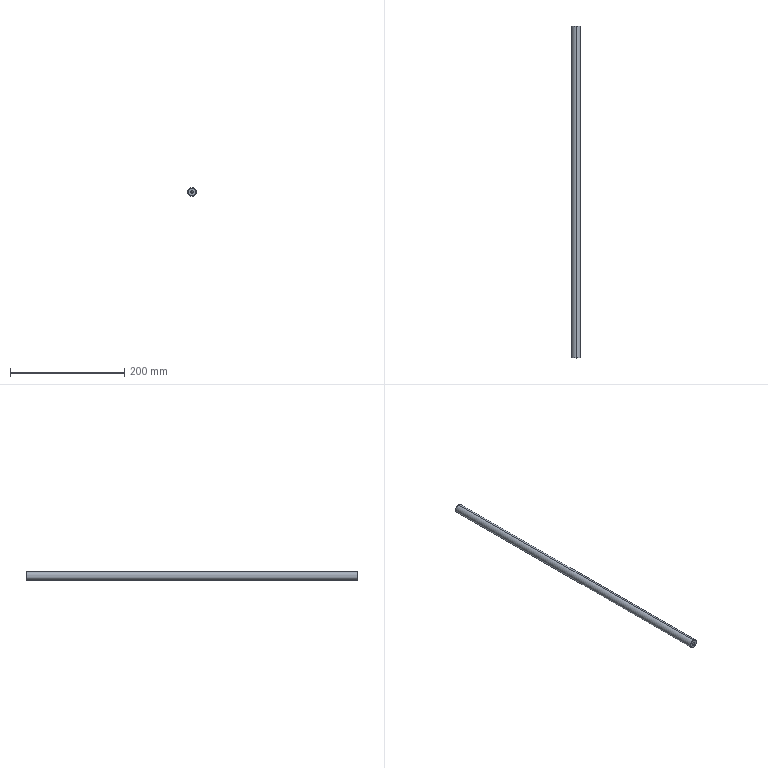Part | STEP file | PN_0005 | 1 solid | 16 faces | box 15 x 580 x 15 mm | volume 101796 mm3 | cone 8 | cylinder 6 | plane 2 | commonest cylinder face diameters 5 x4 15 x2
STEP:
#1=CARTESIAN_POINT('',(0.,0.,0.));
#2=DIRECTION('',(0.,0.,1.));
#3=DIRECTION('',(1.,0.,0.));
#4=AXIS2_PLACEMENT_3D('',#1,#2,#3);
#5=CARTESIAN_POINT('',(0.,580.,7.));
#6=VERTEX_POINT('',#5);
#7=CARTESIAN_POINT('',(0.,580.,-7.));
#8=VERTEX_POINT('',#7);
#9=CARTESIAN_POINT('',(0.,580.,0.));
#10=DIRECTION('',(0.,1.,0.));
#11=DIRECTION('',(0.,0.,1.));
#12=AXIS2_PLACEMENT_3D('',#9,#10,#11);
#13=CIRCLE('',#12,7.);
#14=CARTESIAN_POINT('',(0.,580.,0.));
#15=DIRECTION('',(0.,-1.,0.));
#16=DIRECTION('',(0.,0.,-1.));
#17=AXIS2_PLACEMENT_3D('',#14,#15,#16);
#18=CONICAL_SURFACE('',#17,7.,0.7854);
#19=CARTESIAN_POINT('',(3.142,0.));
#20=DIRECTION('',(-1.,0.));
#21=VECTOR('',#20,1.);
#22=LINE('',#19,#21);
#23=(GEOMETRIC_REPRESENTATION_CONTEXT(2)PARAMETRIC_REPRESENTATION_CONTEXT()REPRESENTATION_CONTEXT('',''));
#24=DEFINITIONAL_REPRESENTATION('',(#22),#23);
#25=PCURVE('',#18,#24);
#26=CARTESIAN_POINT('',(0.,580.,0.));
#27=DIRECTION('',(0.,1.,0.));
#28=DIRECTION('',(0.,0.,1.));
#29=AXIS2_PLACEMENT_3D('',#26,#27,#28);
#30=PLANE('',#29);
#31=CARTESIAN_POINT('',(0.,0.));
#32=DIRECTION('',(1.,0.));
#33=AXIS2_PLACEMENT_2D('',#31,#32);
#34=CIRCLE('',#33,7.);
#35=(GEOMETRIC_REPRESENTATION_CONTEXT(2)PARAMETRIC_REPRESENTATION_CONTEXT()REPRESENTATION_CONTEXT('',''));
#36=DEFINITIONAL_REPRESENTATION('',(#34),#35);
#37=PCURVE('',#30,#36);
#38=SURFACE_CURVE('',#13,(#25,#37),.PCURVE_S1.);
#39=EDGE_CURVE('',#6,#8,#38,.T.);
#40=ORIENTED_EDGE('',*,*,#39,.F.);
#41=CARTESIAN_POINT('',(0.,579.5,7.5));
#42=VERTEX_POINT('',#41);
#43=CARTESIAN_POINT('',(0.,580.,7.));
#44=DIRECTION('',(0.,-0.7071,0.7071));
#45=VECTOR('',#44,1.);
#46=LINE('',#43,#45);
#47=CARTESIAN_POINT('',(3.142,0.));
#48=DIRECTION('',(0.,1.));
#49=VECTOR('',#48,1.);
#50=LINE('',#47,#49);
#51=(GEOMETRIC_REPRESENTATION_CONTEXT(2)PARAMETRIC_REPRESENTATION_CONTEXT()REPRESENTATION_CONTEXT('',''));
#52=DEFINITIONAL_REPRESENTATION('',(#50),#51);
#53=PCURVE('',#18,#52);
#54=CARTESIAN_POINT('',(0.,580.,0.));
#55=DIRECTION('',(0.,-1.,0.));
#56=DIRECTION('',(0.,0.,-1.));
#57=AXIS2_PLACEMENT_3D('',#54,#55,#56);
#58=CONICAL_SURFACE('',#57,7.,0.7854);
#59=CARTESIAN_POINT('',(3.142,0.));
#60=DIRECTION('',(0.,1.));
#61=VECTOR('',#60,1.);
#62=LINE('',#59,#61);
#63=(GEOMETRIC_REPRESENTATION_CONTEXT(2)PARAMETRIC_REPRESENTATION_CONTEXT()REPRESENTATION_CONTEXT('',''));
#64=DEFINITIONAL_REPRESENTATION('',(#62),#63);
#65=PCURVE('',#58,#64);
#66=SURFACE_CURVE('',#46,(#53,#65),.PCURVE_S1.);
#67=EDGE_CURVE('',#6,#42,#66,.T.);
#68=ORIENTED_EDGE('',*,*,#67,.T.);
#69=CARTESIAN_POINT('',(0.,579.5,-7.5));
#70=VERTEX_POINT('',#69);
#71=CARTESIAN_POINT('',(0.,579.5,0.));
#72=DIRECTION('',(0.,-1.,0.));
#73=DIRECTION('',(0.,0.,1.));
#74=AXIS2_PLACEMENT_3D('',#71,#72,#73);
#75=CIRCLE('',#74,7.5);
#76=CARTESIAN_POINT('',(-3.142,0.5));
#77=DIRECTION('',(1.,0.));
#78=VECTOR('',#77,1.);
#79=LINE('',#76,#78);
#80=(GEOMETRIC_REPRESENTATION_CONTEXT(2)PARAMETRIC_REPRESENTATION_CONTEXT()REPRESENTATION_CONTEXT('',''));
#81=DEFINITIONAL_REPRESENTATION('',(#79),#80);
#82=PCURVE('',#18,#81);
#83=CARTESIAN_POINT('',(0.,580.,0.));
#84=DIRECTION('',(0.,-1.,0.));
#85=DIRECTION('',(0.,0.,-1.));
#86=AXIS2_PLACEMENT_3D('',#83,#84,#85);
#87=CYLINDRICAL_SURFACE('',#86,7.5);
#88=CARTESIAN_POINT('',(-3.142,0.5));
#89=DIRECTION('',(1.,0.));
#90=VECTOR('',#89,1.);
#91=LINE('',#88,#90);
#92=(GEOMETRIC_REPRESENTATION_CONTEXT(2)PARAMETRIC_REPRESENTATION_CONTEXT()REPRESENTATION_CONTEXT('',''));
#93=DEFINITIONAL_REPRESENTATION('',(#91),#92);
#94=PCURVE('',#87,#93);
#95=SURFACE_CURVE('',#75,(#82,#94),.PCURVE_S1.);
#96=EDGE_CURVE('',#70,#42,#95,.T.);
#97=ORIENTED_EDGE('',*,*,#96,.F.);
#98=CARTESIAN_POINT('',(0.,580.,-7.));
#99=DIRECTION('',(0.,-0.7071,-0.7071));
#100=VECTOR('',#99,1.);
#101=LINE('',#98,#100);
#102=CARTESIAN_POINT('',(0.,0.));
#103=DIRECTION('',(0.,1.));
#104=VECTOR('',#103,1.);
#105=LINE('',#102,#104);
#106=(GEOMETRIC_REPRESENTATION_CONTEXT(2)PARAMETRIC_REPRESENTATION_CONTEXT()REPRESENTATION_CONTEXT('',''));
#107=DEFINITIONAL_REPRESENTATION('',(#105),#106);
#108=PCURVE('',#18,#107);
#109=CARTESIAN_POINT('',(6.283,0.));
#110=DIRECTION('',(0.,1.));
#111=VECTOR('',#110,1.);
#112=LINE('',#109,#111);
#113=(GEOMETRIC_REPRESENTATION_CONTEXT(2)PARAMETRIC_REPRESENTATION_CONTEXT()REPRESENTATION_CONTEXT('',''));
#114=DEFINITIONAL_REPRESENTATION('',(#112),#113);
#115=PCURVE('',#58,#114);
#116=SURFACE_CURVE('',#101,(#108,#115),.PCURVE_S1.);
#117=EDGE_CURVE('',#8,#70,#116,.T.);
#118=ORIENTED_EDGE('',*,*,#117,.F.);
#119=EDGE_LOOP('',(#40,#68,#97,#118));
#120=FACE_BOUND('',#119,.T.);
#121=ADVANCED_FACE('',(#120),#18,.T.);
#122=CARTESIAN_POINT('',(0.,0.,-7.));
#123=VERTEX_POINT('',#122);
#124=CARTESIAN_POINT('',(0.,0.,7.));
#125=VERTEX_POINT('',#124);
#126=CARTESIAN_POINT('',(0.,0.,0.));
#127=DIRECTION('',(0.,-1.,0.));
#128=DIRECTION('',(0.,0.,1.));
#129=AXIS2_PLACEMENT_3D('',#126,#127,#128);
#130=CIRCLE('',#129,7.);
#131=CARTESIAN_POINT('',(0.,0.5,0.));
#132=DIRECTION('',(0.,1.,0.));
#133=DIRECTION('',(0.,0.,1.));
#134=AXIS2_PLACEMENT_3D('',#131,#132,#133);
#135=CONICAL_SURFACE('',#134,7.5,0.7854);
#136=CARTESIAN_POINT('',(6.283,-0.5));
#137=DIRECTION('',(-1.,0.));
#138=VECTOR('',#137,1.);
#139=LINE('',#136,#138);
#140=(GEOMETRIC_REPRESENTATION_CONTEXT(2)PARAMETRIC_REPRESENTATION_CONTEXT()REPRESENTATION_CONTEXT('',''));
#141=DEFINITIONAL_REPRESENTATION('',(#139),#140);
#142=PCURVE('',#135,#141);
#143=CARTESIAN_POINT('',(0.,0.,0.));
#144=DIRECTION('',(0.,1.,0.));
#145=DIRECTION('',(0.,0.,1.));
#146=AXIS2_PLACEMENT_3D('',#143,#144,#145);
#147=PLANE('',#146);
#148=CARTESIAN_POINT('',(7.,0.));
#149=CARTESIAN_POINT('',(7.,-12.124));
#150=CARTESIAN_POINT('',(-3.5,-6.062));
#151=CARTESIAN_POINT('',(-14.,0.));
#152=CARTESIAN_POINT('',(-3.5,6.062));
#153=CARTESIAN_POINT('',(7.,12.124));
#154=CARTESIAN_POINT('',(7.,0.));
#155=(BOUNDED_CURVE()B_SPLINE_CURVE(2,(#148,#149,#150,#151,#152,#153,#154),.UNSPECIFIED.,.T.,.F.)B_SPLINE_CURVE_WITH_KNOTS((1,2,2,2,2,1),(-2.094,0.,2.094,4.189,6.283,8.378),.UNSPECIFIED.)CURVE()GEOMETRIC_REPRESENTATION_ITEM()RATIONAL_B_SPLINE_CURVE((1.,0.5,1.,0.5,1.,0.5,1.))REPRESENTATION_ITEM(''));
#156=(GEOMETRIC_REPRESENTATION_CONTEXT(2)PARAMETRIC_REPRESENTATION_CONTEXT()REPRESENTATION_CONTEXT('',''));
#157=DEFINITIONAL_REPRESENTATION('',(#155),#156);
#158=PCURVE('',#147,#157);
#159=SURFACE_CURVE('',#130,(#142,#158),.PCURVE_S1.);
#160=EDGE_CURVE('',#123,#125,#159,.T.);
#161=ORIENTED_EDGE('',*,*,#160,.F.);
#162=CARTESIAN_POINT('',(0.,0.5,-7.5));
#163=VERTEX_POINT('',#162);
#164=CARTESIAN_POINT('',(0.,0.5,-7.5));
#165=DIRECTION('',(0.,0.7071,-0.7071));
#166=VECTOR('',#165,1.);
#167=LINE('',#164,#166);
#168=CARTESIAN_POINT('',(3.142,0.));
#169=DIRECTION('',(0.,1.));
#170=VECTOR('',#169,1.);
#171=LINE('',#168,#170);
#172=(GEOMETRIC_REPRESENTATION_CONTEXT(2)PARAMETRIC_REPRESENTATION_CONTEXT()REPRESENTATION_CONTEXT('',''));
#173=DEFINITIONAL_REPRESENTATION('',(#171),#172);
#174=PCURVE('',#135,#173);
#175=CARTESIAN_POINT('',(0.,0.5,0.));
#176=DIRECTION('',(0.,1.,0.));
#177=DIRECTION('',(0.,0.,1.));
#178=AXIS2_PLACEMENT_3D('',#175,#176,#177);
#179=CONICAL_SURFACE('',#178,7.5,0.7854);
#180=CARTESIAN_POINT('',(3.142,0.));
#181=DIRECTION('',(0.,1.));
#182=VECTOR('',#181,1.);
#183=LINE('',#180,#182);
#184=(GEOMETRIC_REPRESENTATION_CONTEXT(2)PARAMETRIC_REPRESENTATION_CONTEXT()REPRESENTATION_CONTEXT('',''));
#185=DEFINITIONAL_REPRESENTATION('',(#183),#184);
#186=PCURVE('',#179,#185);
#187=SURFACE_CURVE('',#167,(#174,#186),.PCURVE_S1.);
#188=EDGE_CURVE('',#123,#163,#187,.T.);
#189=ORIENTED_EDGE('',*,*,#188,.T.);
#190=CARTESIAN_POINT('',(0.,0.5,7.5));
#191=VERTEX_POINT('',#190);
#192=CARTESIAN_POINT('',(0.,0.5,0.));
#193=DIRECTION('',(0.,1.,0.));
#194=DIRECTION('',(0.,0.,1.));
#195=AXIS2_PLACEMENT_3D('',#192,#193,#194);
#196=CIRCLE('',#195,7.5);
#197=CARTESIAN_POINT('',(0.,0.));
#198=DIRECTION('',(1.,0.));
#199=VECTOR('',#198,1.);
#200=LINE('',#197,#199);
#201=(GEOMETRIC_REPRESENTATION_CONTEXT(2)PARAMETRIC_REPRESENTATION_CONTEXT()REPRESENTATION_CONTEXT('',''));
#202=DEFINITIONAL_REPRESENTATION('',(#200),#201);
#203=PCURVE('',#135,#202);
#204=CARTESIAN_POINT('',(3.142,579.5));
#205=DIRECTION('',(-1.,0.));
#206=VECTOR('',#205,1.);
#207=LINE('',#204,#206);
#208=(GEOMETRIC_REPRESENTATION_CONTEXT(2)PARAMETRIC_REPRESENTATION_CONTEXT()REPRESENTATION_CONTEXT('',''));
#209=DEFINITIONAL_REPRESENTATION('',(#207),#208);
#210=PCURVE('',#87,#209);
#211=SURFACE_CURVE('',#196,(#203,#210),.PCURVE_S1.);
#212=EDGE_CURVE('',#191,#163,#211,.T.);
#213=ORIENTED_EDGE('',*,*,#212,.F.);
#214=CARTESIAN_POINT('',(0.,0.5,7.5));
#215=DIRECTION('',(0.,0.7071,0.7071));
#216=VECTOR('',#215,1.);
#217=LINE('',#214,#216);
#218=CARTESIAN_POINT('',(0.,0.));
#219=DIRECTION('',(0.,1.));
#220=VECTOR('',#219,1.);
#221=LINE('',#218,#220);
#222=(GEOMETRIC_REPRESENTATION_CONTEXT(2)PARAMETRIC_REPRESENTATION_CONTEXT()REPRESENTATION_CONTEXT('',''));
#223=DEFINITIONAL_REPRESENTATION('',(#221),#222);
#224=PCURVE('',#135,#223);
#225=CARTESIAN_POINT('',(6.283,0.));
#226=DIRECTION('',(0.,1.));
#227=VECTOR('',#226,1.);
#228=LINE('',#225,#227);
#229=(GEOMETRIC_REPRESENTATION_CONTEXT(2)PARAMETRIC_REPRESENTATION_CONTEXT()REPRESENTATION_CONTEXT('',''));
#230=DEFINITIONAL_REPRESENTATION('',(#228),#229);
#231=PCURVE('',#179,#230);
#232=SURFACE_CURVE('',#217,(#224,#231),.PCURVE_S1.);
#233=EDGE_CURVE('',#125,#191,#232,.T.);
#234=ORIENTED_EDGE('',*,*,#233,.F.);
#235=EDGE_LOOP('',(#161,#189,#213,#234));
#236=FACE_BOUND('',#235,.T.);
#237=ADVANCED_FACE('',(#236),#135,.T.);
#238=CARTESIAN_POINT('',(0.,563.,2.5));
#239=VERTEX_POINT('',#238);
#240=CARTESIAN_POINT('',(0.,580.,2.5));
#241=VERTEX_POINT('',#240);
#242=CARTESIAN_POINT('',(0.,580.,2.5));
#243=DIRECTION('',(0.,1.,0.));
#244=VECTOR('',#243,1.);
#245=LINE('',#242,#244);
#246=CARTESIAN_POINT('',(0.,580.,0.));
#247=DIRECTION('',(0.,1.,0.));
#248=DIRECTION('',(0.,0.,1.));
#249=AXIS2_PLACEMENT_3D('',#246,#247,#248);
#250=CYLINDRICAL_SURFACE('',#249,2.5);
#251=CARTESIAN_POINT('',(6.283,0.));
#252=DIRECTION('',(0.,1.));
#253=VECTOR('',#252,1.);
#254=LINE('',#251,#253);
#255=(GEOMETRIC_REPRESENTATION_CONTEXT(2)PARAMETRIC_REPRESENTATION_CONTEXT()REPRESENTATION_CONTEXT('',''));
#256=DEFINITIONAL_REPRESENTATION('',(#254),#255);
#257=PCURVE('',#250,#256);
#258=CARTESIAN_POINT('',(0.,580.,0.));
#259=DIRECTION('',(0.,1.,0.));
#260=DIRECTION('',(0.,0.,1.));
#261=AXIS2_PLACEMENT_3D('',#258,#259,#260);
#262=CYLINDRICAL_SURFACE('',#261,2.5);
#263=CARTESIAN_POINT('',(0.,0.));
#264=DIRECTION('',(0.,1.));
#265=VECTOR('',#264,1.);
#266=LINE('',#263,#265);
#267=(GEOMETRIC_REPRESENTATION_CONTEXT(2)PARAMETRIC_REPRESENTATION_CONTEXT()REPRESENTATION_CONTEXT('',''));
#268=DEFINITIONAL_REPRESENTATION('',(#266),#267);
#269=PCURVE('',#262,#268);
#270=SURFACE_CURVE('',#245,(#257,#269),.PCURVE_S1.);
#271=EDGE_CURVE('',#239,#241,#270,.T.);
#272=ORIENTED_EDGE('',*,*,#271,.T.);
#273=CARTESIAN_POINT('',(0.,580.,-2.5));
#274=VERTEX_POINT('',#273);
#275=CARTESIAN_POINT('',(0.,580.,0.));
#276=DIRECTION('',(0.,1.,0.));
#277=DIRECTION('',(0.,0.,1.));
#278=AXIS2_PLACEMENT_3D('',#275,#276,#277);
#279=CIRCLE('',#278,2.5);
#280=CARTESIAN_POINT('',(0.,0.));
#281=DIRECTION('',(1.,0.));
#282=VECTOR('',#281,1.);
#283=LINE('',#280,#282);
#284=(GEOMETRIC_REPRESENTATION_CONTEXT(2)PARAMETRIC_REPRESENTATION_CONTEXT()REPRESENTATION_CONTEXT('',''));
#285=DEFINITIONAL_REPRESENTATION('',(#283),#284);
#286=PCURVE('',#250,#285);
#287=CARTESIAN_POINT('',(0.,0.));
#288=DIRECTION('',(1.,0.));
#289=AXIS2_PLACEMENT_2D('',#287,#288);
#290=CIRCLE('',#289,2.5);
#291=(GEOMETRIC_REPRESENTATION_CONTEXT(2)PARAMETRIC_REPRESENTATION_CONTEXT()REPRESENTATION_CONTEXT('',''));
#292=DEFINITIONAL_REPRESENTATION('',(#290),#291);
#293=PCURVE('',#30,#292);
#294=SURFACE_CURVE('',#279,(#286,#293),.PCURVE_S1.);
#295=EDGE_CURVE('',#274,#241,#294,.T.);
#296=ORIENTED_EDGE('',*,*,#295,.F.);
#297=CARTESIAN_POINT('',(0.,563.,-2.5));
#298=VERTEX_POINT('',#297);
#299=CARTESIAN_POINT('',(0.,580.,-2.5));
#300=DIRECTION('',(0.,1.,0.));
#301=VECTOR('',#300,1.);
#302=LINE('',#299,#301);
#303=CARTESIAN_POINT('',(3.142,0.));
#304=DIRECTION('',(0.,1.));
#305=VECTOR('',#304,1.);
#306=LINE('',#303,#305);
#307=(GEOMETRIC_REPRESENTATION_CONTEXT(2)PARAMETRIC_REPRESENTATION_CONTEXT()REPRESENTATION_CONTEXT('',''));
#308=DEFINITIONAL_REPRESENTATION('',(#306),#307);
#309=PCURVE('',#250,#308);
#310=CARTESIAN_POINT('',(3.142,0.));
#311=DIRECTION('',(0.,1.));
#312=VECTOR('',#311,1.);
#313=LINE('',#310,#312);
#314=(GEOMETRIC_REPRESENTATION_CONTEXT(2)PARAMETRIC_REPRESENTATION_CONTEXT()REPRESENTATION_CONTEXT('',''));
#315=DEFINITIONAL_REPRESENTATION('',(#313),#314);
#316=PCURVE('',#262,#315);
#317=SURFACE_CURVE('',#302,(#309,#316),.PCURVE_S1.);
#318=EDGE_CURVE('',#298,#274,#317,.T.);
#319=ORIENTED_EDGE('',*,*,#318,.F.);
#320=CARTESIAN_POINT('',(0.,563.,0.));
#321=DIRECTION('',(0.,1.,0.));
#322=DIRECTION('',(0.,0.,1.));
#323=AXIS2_PLACEMENT_3D('',#320,#321,#322);
#324=CIRCLE('',#323,2.5);
#325=CARTESIAN_POINT('',(0.,-17.));
#326=DIRECTION('',(1.,0.));
#327=VECTOR('',#326,1.);
#328=LINE('',#325,#327);
#329=(GEOMETRIC_REPRESENTATION_CONTEXT(2)PARAMETRIC_REPRESENTATION_CONTEXT()REPRESENTATION_CONTEXT('',''));
#330=DEFINITIONAL_REPRESENTATION('',(#328),#329);
#331=PCURVE('',#250,#330);
#332=CARTESIAN_POINT('',(0.,563.,0.));
#333=DIRECTION('',(0.,1.,0.));
#334=DIRECTION('',(0.,0.,1.));
#335=AXIS2_PLACEMENT_3D('',#332,#333,#334);
#336=CONICAL_SURFACE('',#335,2.5,1.03);
#337=CARTESIAN_POINT('',(0.,0.));
#338=DIRECTION('',(1.,0.));
#339=VECTOR('',#338,1.);
#340=LINE('',#337,#339);
#341=(GEOMETRIC_REPRESENTATION_CONTEXT(2)PARAMETRIC_REPRESENTATION_CONTEXT()REPRESENTATION_CONTEXT('',''));
#342=DEFINITIONAL_REPRESENTATION('',(#340),#341);
#343=PCURVE('',#336,#342);
#344=SURFACE_CURVE('',#324,(#331,#343),.PCURVE_S1.);
#345=EDGE_CURVE('',#298,#239,#344,.T.);
#346=ORIENTED_EDGE('',*,*,#345,.T.);
#347=EDGE_LOOP('',(#272,#296,#319,#346));
#348=FACE_BOUND('',#347,.F.);
#349=ADVANCED_FACE('',(#348),#250,.F.);
#350=ORIENTED_EDGE('',*,*,#345,.F.);
#351=CARTESIAN_POINT('',(0.,561.498,0.));
#352=VERTEX_POINT('',#351);
#353=CARTESIAN_POINT('',(0.,563.,-2.5));
#354=DIRECTION('',(0.,0.515,-0.8572));
#355=VECTOR('',#354,1.);
#356=LINE('',#353,#355);
#357=CARTESIAN_POINT('',(3.142,-1.502));
#358=CARTESIAN_POINT('',(3.142,-1.479));
#359=CARTESIAN_POINT('',(3.142,-1.434));
#360=CARTESIAN_POINT('',(3.142,-1.366));
#361=CARTESIAN_POINT('',(3.142,-1.297));
#362=CARTESIAN_POINT('',(3.142,-1.229));
#363=CARTESIAN_POINT('',(3.142,-1.161));
#364=CARTESIAN_POINT('',(3.142,-1.092));
#365=CARTESIAN_POINT('',(3.142,-1.024));
#366=CARTESIAN_POINT('',(3.142,-0.9559));
#367=CARTESIAN_POINT('',(3.142,-0.8876));
#368=CARTESIAN_POINT('',(3.142,-0.8194));
#369=CARTESIAN_POINT('',(3.142,-0.7511));
#370=CARTESIAN_POINT('',(3.142,-0.6828));
#371=CARTESIAN_POINT('',(3.142,-0.6145));
#372=CARTESIAN_POINT('',(3.142,-0.5462));
#373=CARTESIAN_POINT('',(3.142,-0.478));
#374=CARTESIAN_POINT('',(3.142,-0.4097));
#375=CARTESIAN_POINT('',(3.142,-0.3414));
#376=CARTESIAN_POINT('',(3.142,-0.2731));
#377=CARTESIAN_POINT('',(3.142,-0.2048));
#378=CARTESIAN_POINT('',(3.142,-0.1366));
#379=CARTESIAN_POINT('',(3.142,-0.06828));
#380=CARTESIAN_POINT('',(3.142,-0.02276));
#381=CARTESIAN_POINT('',(3.142,0.));
#382=B_SPLINE_CURVE_WITH_KNOTS('',3,(#357,#358,#359,#360,#361,#362,#363,#364,#365,#366,#367,#368,#369,#370,#371,#372,#373,#374,#375,#376,#377,#378,#379,#380,#381),.UNSPECIFIED.,.F.,.F.,(4,1,1,1,1,1,1,1,1,1,1,1,1,1,1,1,1,1,1,1,1,1,4),(-2.917,-2.784,-2.651,-2.519,-2.386,-2.254,-2.121,-1.989,-1.856,-1.723,-1.591,-1.458,-1.326,-1.193,-1.061,-0.928,-0.7954,-0.6629,-0.5303,-0.3977,-0.2651,-0.1326,0.),.UNSPECIFIED.);
#383=(GEOMETRIC_REPRESENTATION_CONTEXT(2)PARAMETRIC_REPRESENTATION_CONTEXT()REPRESENTATION_CONTEXT('',''));
#384=DEFINITIONAL_REPRESENTATION('',(#382),#383);
#385=PCURVE('',#336,#384);
#386=CARTESIAN_POINT('',(0.,563.,0.));
#387=DIRECTION('',(0.,1.,0.));
#388=DIRECTION('',(0.,0.,1.));
#389=AXIS2_PLACEMENT_3D('',#386,#387,#388);
#390=CONICAL_SURFACE('',#389,2.5,1.03);
#391=CARTESIAN_POINT('',(3.142,-1.502));
#392=CARTESIAN_POINT('',(3.142,-1.479));
#393=CARTESIAN_POINT('',(3.142,-1.434));
#394=CARTESIAN_POINT('',(3.142,-1.366));
#395=CARTESIAN_POINT('',(3.142,-1.297));
#396=CARTESIAN_POINT('',(3.142,-1.229));
#397=CARTESIAN_POINT('',(3.142,-1.161));
#398=CARTESIAN_POINT('',(3.142,-1.092));
#399=CARTESIAN_POINT('',(3.142,-1.024));
#400=CARTESIAN_POINT('',(3.142,-0.9559));
#401=CARTESIAN_POINT('',(3.142,-0.8876));
#402=CARTESIAN_POINT('',(3.142,-0.8194));
#403=CARTESIAN_POINT('',(3.142,-0.7511));
#404=CARTESIAN_POINT('',(3.142,-0.6828));
#405=CARTESIAN_POINT('',(3.142,-0.6145));
#406=CARTESIAN_POINT('',(3.142,-0.5462));
#407=CARTESIAN_POINT('',(3.142,-0.478));
#408=CARTESIAN_POINT('',(3.142,-0.4097));
#409=CARTESIAN_POINT('',(3.142,-0.3414));
#410=CARTESIAN_POINT('',(3.142,-0.2731));
#411=CARTESIAN_POINT('',(3.142,-0.2048));
#412=CARTESIAN_POINT('',(3.142,-0.1366));
#413=CARTESIAN_POINT('',(3.142,-0.06828));
#414=CARTESIAN_POINT('',(3.142,-0.02276));
#415=CARTESIAN_POINT('',(3.142,0.));
#416=B_SPLINE_CURVE_WITH_KNOTS('',3,(#391,#392,#393,#394,#395,#396,#397,#398,#399,#400,#401,#402,#403,#404,#405,#406,#407,#408,#409,#410,#411,#412,#413,#414,#415),.UNSPECIFIED.,.F.,.F.,(4,1,1,1,1,1,1,1,1,1,1,1,1,1,1,1,1,1,1,1,1,1,4),(-2.917,-2.784,-2.651,-2.519,-2.386,-2.254,-2.121,-1.989,-1.856,-1.723,-1.591,-1.458,-1.326,-1.193,-1.061,-0.928,-0.7954,-0.6629,-0.5303,-0.3977,-0.2651,-0.1326,0.),.UNSPECIFIED.);
#417=(GEOMETRIC_REPRESENTATION_CONTEXT(2)PARAMETRIC_REPRESENTATION_CONTEXT()REPRESENTATION_CONTEXT('',''));
#418=DEFINITIONAL_REPRESENTATION('',(#416),#417);
#419=PCURVE('',#390,#418);
#420=SURFACE_CURVE('',#356,(#385,#419),.PCURVE_S1.);
#421=EDGE_CURVE('',#352,#298,#420,.T.);
#422=ORIENTED_EDGE('',*,*,#421,.F.);
#423=CARTESIAN_POINT('',(0.,563.,2.5));
#424=DIRECTION('',(0.,0.515,0.8572));
#425=VECTOR('',#424,1.);
#426=LINE('',#423,#425);
#427=CARTESIAN_POINT('',(6.283,-1.502));
#428=CARTESIAN_POINT('',(6.283,-1.479));
#429=CARTESIAN_POINT('',(6.283,-1.434));
#430=CARTESIAN_POINT('',(6.283,-1.366));
#431=CARTESIAN_POINT('',(6.283,-1.297));
#432=CARTESIAN_POINT('',(6.283,-1.229));
#433=CARTESIAN_POINT('',(6.283,-1.161));
#434=CARTESIAN_POINT('',(6.283,-1.092));
#435=CARTESIAN_POINT('',(6.283,-1.024));
#436=CARTESIAN_POINT('',(6.283,-0.9559));
#437=CARTESIAN_POINT('',(6.283,-0.8876));
#438=CARTESIAN_POINT('',(6.283,-0.8194));
#439=CARTESIAN_POINT('',(6.283,-0.7511));
#440=CARTESIAN_POINT('',(6.283,-0.6828));
#441=CARTESIAN_POINT('',(6.283,-0.6145));
#442=CARTESIAN_POINT('',(6.283,-0.5462));
#443=CARTESIAN_POINT('',(6.283,-0.478));
#444=CARTESIAN_POINT('',(6.283,-0.4097));
#445=CARTESIAN_POINT('',(6.283,-0.3414));
#446=CARTESIAN_POINT('',(6.283,-0.2731));
#447=CARTESIAN_POINT('',(6.283,-0.2048));
#448=CARTESIAN_POINT('',(6.283,-0.1366));
#449=CARTESIAN_POINT('',(6.283,-0.06828));
#450=CARTESIAN_POINT('',(6.283,-0.02276));
#451=CARTESIAN_POINT('',(6.283,0.));
#452=B_SPLINE_CURVE_WITH_KNOTS('',3,(#427,#428,#429,#430,#431,#432,#433,#434,#435,#436,#437,#438,#439,#440,#441,#442,#443,#444,#445,#446,#447,#448,#449,#450,#451),.UNSPECIFIED.,.F.,.F.,(4,1,1,1,1,1,1,1,1,1,1,1,1,1,1,1,1,1,1,1,1,1,4),(-2.917,-2.784,-2.651,-2.519,-2.386,-2.254,-2.121,-1.989,-1.856,-1.723,-1.591,-1.458,-1.326,-1.193,-1.061,-0.928,-0.7954,-0.6629,-0.5303,-0.3977,-0.2651,-0.1326,0.),.UNSPECIFIED.);
#453=(GEOMETRIC_REPRESENTATION_CONTEXT(2)PARAMETRIC_REPRESENTATION_CONTEXT()REPRESENTATION_CONTEXT('',''));
#454=DEFINITIONAL_REPRESENTATION('',(#452),#453);
#455=PCURVE('',#336,#454);
#456=CARTESIAN_POINT('',(0.,-1.502));
#457=CARTESIAN_POINT('',(0.,-1.479));
#458=CARTESIAN_POINT('',(0.,-1.434));
#459=CARTESIAN_POINT('',(0.,-1.366));
#460=CARTESIAN_POINT('',(0.,-1.297));
#461=CARTESIAN_POINT('',(0.,-1.229));
#462=CARTESIAN_POINT('',(0.,-1.161));
#463=CARTESIAN_POINT('',(0.,-1.092));
#464=CARTESIAN_POINT('',(0.,-1.024));
#465=CARTESIAN_POINT('',(0.,-0.9559));
#466=CARTESIAN_POINT('',(0.,-0.8876));
#467=CARTESIAN_POINT('',(0.,-0.8194));
#468=CARTESIAN_POINT('',(0.,-0.7511));
#469=CARTESIAN_POINT('',(0.,-0.6828));
#470=CARTESIAN_POINT('',(0.,-0.6145));
#471=CARTESIAN_POINT('',(0.,-0.5462));
#472=CARTESIAN_POINT('',(0.,-0.478));
#473=CARTESIAN_POINT('',(0.,-0.4097));
#474=CARTESIAN_POINT('',(0.,-0.3414));
#475=CARTESIAN_POINT('',(0.,-0.2731));
#476=CARTESIAN_POINT('',(0.,-0.2048));
#477=CARTESIAN_POINT('',(0.,-0.1366));
#478=CARTESIAN_POINT('',(0.,-0.06828));
#479=CARTESIAN_POINT('',(0.,-0.02276));
#480=CARTESIAN_POINT('',(0.,0.));
#481=B_SPLINE_CURVE_WITH_KNOTS('',3,(#456,#457,#458,#459,#460,#461,#462,#463,#464,#465,#466,#467,#468,#469,#470,#471,#472,#473,#474,#475,#476,#477,#478,#479,#480),.UNSPECIFIED.,.F.,.F.,(4,1,1,1,1,1,1,1,1,1,1,1,1,1,1,1,1,1,1,1,1,1,4),(-2.917,-2.784,-2.651,-2.519,-2.386,-2.254,-2.121,-1.989,-1.856,-1.723,-1.591,-1.458,-1.326,-1.193,-1.061,-0.928,-0.7954,-0.6629,-0.5303,-0.3977,-0.2651,-0.1326,0.),.UNSPECIFIED.);
#482=(GEOMETRIC_REPRESENTATION_CONTEXT(2)PARAMETRIC_REPRESENTATION_CONTEXT()REPRESENTATION_CONTEXT('',''));
#483=DEFINITIONAL_REPRESENTATION('',(#481),#482);
#484=PCURVE('',#390,#483);
#485=SURFACE_CURVE('',#426,(#455,#484),.PCURVE_S1.);
#486=EDGE_CURVE('',#352,#239,#485,.T.);
#487=ORIENTED_EDGE('',*,*,#486,.T.);
#488=EDGE_LOOP('',(#350,#422,#487));
#489=FACE_BOUND('',#488,.F.);
#490=ADVANCED_FACE('',(#489),#336,.F.);
#491=CARTESIAN_POINT('',(0.,17.,-2.5));
#492=VERTEX_POINT('',#491);
#493=CARTESIAN_POINT('',(0.,0.,-2.5));
#494=VERTEX_POINT('',#493);
#495=CARTESIAN_POINT('',(0.,0.,-2.5));
#496=DIRECTION('',(0.,-1.,0.));
#497=VECTOR('',#496,1.);
#498=LINE('',#495,#497);
#499=CARTESIAN_POINT('',(0.,0.,0.));
#500=DIRECTION('',(0.,-1.,0.));
#501=DIRECTION('',(0.,0.,-1.));
#502=AXIS2_PLACEMENT_3D('',#499,#500,#501);
#503=CYLINDRICAL_SURFACE('',#502,2.5);
#504=CARTESIAN_POINT('',(6.283,0.));
#505=DIRECTION('',(0.,1.));
#506=VECTOR('',#505,1.);
#507=LINE('',#504,#506);
#508=(GEOMETRIC_REPRESENTATION_CONTEXT(2)PARAMETRIC_REPRESENTATION_CONTEXT()REPRESENTATION_CONTEXT('',''));
#509=DEFINITIONAL_REPRESENTATION('',(#507),#508);
#510=PCURVE('',#503,#509);
#511=CARTESIAN_POINT('',(0.,0.,0.));
#512=DIRECTION('',(0.,-1.,0.));
#513=DIRECTION('',(0.,0.,-1.));
#514=AXIS2_PLACEMENT_3D('',#511,#512,#513);
#515=CYLINDRICAL_SURFACE('',#514,2.5);
#516=CARTESIAN_POINT('',(0.,0.));
#517=DIRECTION('',(0.,1.));
#518=VECTOR('',#517,1.);
#519=LINE('',#516,#518);
#520=(GEOMETRIC_REPRESENTATION_CONTEXT(2)PARAMETRIC_REPRESENTATION_CONTEXT()REPRESENTATION_CONTEXT('',''));
#521=DEFINITIONAL_REPRESENTATION('',(#519),#520);
#522=PCURVE('',#515,#521);
#523=SURFACE_CURVE('',#498,(#510,#522),.PCURVE_S1.);
#524=EDGE_CURVE('',#492,#494,#523,.T.);
#525=ORIENTED_EDGE('',*,*,#524,.T.);
#526=CARTESIAN_POINT('',(0.,0.,2.5));
#527=VERTEX_POINT('',#526);
#528=CARTESIAN_POINT('',(0.,0.,0.));
#529=DIRECTION('',(0.,-1.,0.));
#530=DIRECTION('',(0.,0.,-1.));
#531=AXIS2_PLACEMENT_3D('',#528,#529,#530);
#532=CIRCLE('',#531,2.5);
#533=CARTESIAN_POINT('',(0.,0.));
#534=DIRECTION('',(1.,0.));
#535=VECTOR('',#534,1.);
#536=LINE('',#533,#535);
#537=(GEOMETRIC_REPRESENTATION_CONTEXT(2)PARAMETRIC_REPRESENTATION_CONTEXT()REPRESENTATION_CONTEXT('',''));
#538=DEFINITIONAL_REPRESENTATION('',(#536),#537);
#539=PCURVE('',#503,#538);
#540=CARTESIAN_POINT('',(-2.5,0.));
#541=CARTESIAN_POINT('',(-2.5,4.33));
#542=CARTESIAN_POINT('',(1.25,2.165));
#543=CARTESIAN_POINT('',(5.,0.));
#544=CARTESIAN_POINT('',(1.25,-2.165));
#545=CARTESIAN_POINT('',(-2.5,-4.33));
#546=CARTESIAN_POINT('',(-2.5,0.));
#547=(BOUNDED_CURVE()B_SPLINE_CURVE(2,(#540,#541,#542,#543,#544,#545,#546),.UNSPECIFIED.,.T.,.F.)B_SPLINE_CURVE_WITH_KNOTS((1,2,2,2,2,1),(-2.094,0.,2.094,4.189,6.283,8.378),.UNSPECIFIED.)CURVE()GEOMETRIC_REPRESENTATION_ITEM()RATIONAL_B_SPLINE_CURVE((1.,0.5,1.,0.5,1.,0.5,1.))REPRESENTATION_ITEM(''));
#548=(GEOMETRIC_REPRESENTATION_CONTEXT(2)PARAMETRIC_REPRESENTATION_CONTEXT()REPRESENTATION_CONTEXT('',''));
#549=DEFINITIONAL_REPRESENTATION('',(#547),#548);
#550=PCURVE('',#147,#549);
#551=SURFACE_CURVE('',#532,(#539,#550),.PCURVE_S1.);
#552=EDGE_CURVE('',#527,#494,#551,.T.);
#553=ORIENTED_EDGE('',*,*,#552,.F.);
#554=CARTESIAN_POINT('',(0.,17.,2.5));
#555=VERTEX_POINT('',#554);
#556=CARTESIAN_POINT('',(0.,0.,2.5));
#557=DIRECTION('',(0.,-1.,0.));
#558=VECTOR('',#557,1.);
#559=LINE('',#556,#558);
#560=CARTESIAN_POINT('',(3.142,0.));
#561=DIRECTION('',(0.,1.));
#562=VECTOR('',#561,1.);
#563=LINE('',#560,#562);
#564=(GEOMETRIC_REPRESENTATION_CONTEXT(2)PARAMETRIC_REPRESENTATION_CONTEXT()REPRESENTATION_CONTEXT('',''));
#565=DEFINITIONAL_REPRESENTATION('',(#563),#564);
#566=PCURVE('',#503,#565);
#567=CARTESIAN_POINT('',(3.142,0.));
#568=DIRECTION('',(0.,1.));
#569=VECTOR('',#568,1.);
#570=LINE('',#567,#569);
#571=(GEOMETRIC_REPRESENTATION_CONTEXT(2)PARAMETRIC_REPRESENTATION_CONTEXT()REPRESENTATION_CONTEXT('',''));
#572=DEFINITIONAL_REPRESENTATION('',(#570),#571);
#573=PCURVE('',#515,#572);
#574=SURFACE_CURVE('',#559,(#566,#573),.PCURVE_S1.);
#575=EDGE_CURVE('',#555,#527,#574,.T.);
#576=ORIENTED_EDGE('',*,*,#575,.F.);
#577=CARTESIAN_POINT('',(0.,17.,0.));
#578=DIRECTION('',(0.,-1.,0.));
#579=DIRECTION('',(0.,0.,-1.));
#580=AXIS2_PLACEMENT_3D('',#577,#578,#579);
#581=CIRCLE('',#580,2.5);
#582=CARTESIAN_POINT('',(0.,-17.));
#583=DIRECTION('',(1.,0.));
#584=VECTOR('',#583,1.);
#585=LINE('',#582,#584);
#586=(GEOMETRIC_REPRESENTATION_CONTEXT(2)PARAMETRIC_REPRESENTATION_CONTEXT()REPRESENTATION_CONTEXT('',''));
#587=DEFINITIONAL_REPRESENTATION('',(#585),#586);
#588=PCURVE('',#503,#587);
#589=CARTESIAN_POINT('',(0.,17.,0.));
#590=DIRECTION('',(0.,-1.,0.));
#591=DIRECTION('',(0.,0.,-1.));
#592=AXIS2_PLACEMENT_3D('',#589,#590,#591);
#593=CONICAL_SURFACE('',#592,2.5,1.03);
#594=CARTESIAN_POINT('',(0.,0.));
#595=DIRECTION('',(1.,0.));
#596=VECTOR('',#595,1.);
#597=LINE('',#594,#596);
#598=(GEOMETRIC_REPRESENTATION_CONTEXT(2)PARAMETRIC_REPRESENTATION_CONTEXT()REPRESENTATION_CONTEXT('',''));
#599=DEFINITIONAL_REPRESENTATION('',(#597),#598);
#600=PCURVE('',#593,#599);
#601=SURFACE_CURVE('',#581,(#588,#600),.PCURVE_S1.);
#602=EDGE_CURVE('',#555,#492,#601,.T.);
#603=ORIENTED_EDGE('',*,*,#602,.T.);
#604=EDGE_LOOP('',(#525,#553,#576,#603));
#605=FACE_BOUND('',#604,.F.);
#606=ADVANCED_FACE('',(#605),#503,.F.);
#607=ORIENTED_EDGE('',*,*,#602,.F.);
#608=CARTESIAN_POINT('',(0.,18.502,0.));
#609=VERTEX_POINT('',#608);
#610=CARTESIAN_POINT('',(0.,17.,2.5));
#611=DIRECTION('',(0.,-0.515,0.8572));
#612=VECTOR('',#611,1.);
#613=LINE('',#610,#612);
#614=CARTESIAN_POINT('',(3.142,0.));
#615=DIRECTION('',(0.,1.));
#616=VECTOR('',#615,1.);
#617=LINE('',#614,#616);
#618=(GEOMETRIC_REPRESENTATION_CONTEXT(2)PARAMETRIC_REPRESENTATION_CONTEXT()REPRESENTATION_CONTEXT('',''));
#619=DEFINITIONAL_REPRESENTATION('',(#617),#618);
#620=PCURVE('',#593,#619);
#621=CARTESIAN_POINT('',(0.,17.,0.));
#622=DIRECTION('',(0.,-1.,0.));
#623=DIRECTION('',(0.,0.,-1.));
#624=AXIS2_PLACEMENT_3D('',#621,#622,#623);
#625=CONICAL_SURFACE('',#624,2.5,1.03);
#626=CARTESIAN_POINT('',(3.142,0.));
#627=DIRECTION('',(0.,1.));
#628=VECTOR('',#627,1.);
#629=LINE('',#626,#628);
#630=(GEOMETRIC_REPRESENTATION_CONTEXT(2)PARAMETRIC_REPRESENTATION_CONTEXT()REPRESENTATION_CONTEXT('',''));
#631=DEFINITIONAL_REPRESENTATION('',(#629),#630);
#632=PCURVE('',#625,#631);
#633=SURFACE_CURVE('',#613,(#620,#632),.PCURVE_S1.);
#634=EDGE_CURVE('',#609,#555,#633,.T.);
#635=ORIENTED_EDGE('',*,*,#634,.F.);
#636=CARTESIAN_POINT('',(0.,17.,-2.5));
#637=DIRECTION('',(0.,-0.515,-0.8572));
#638=VECTOR('',#637,1.);
#639=LINE('',#636,#638);
#640=CARTESIAN_POINT('',(6.283,0.));
#641=DIRECTION('',(0.,1.));
#642=VECTOR('',#641,1.);
#643=LINE('',#640,#642);
#644=(GEOMETRIC_REPRESENTATION_CONTEXT(2)PARAMETRIC_REPRESENTATION_CONTEXT()REPRESENTATION_CONTEXT('',''));
#645=DEFINITIONAL_REPRESENTATION('',(#643),#644);
#646=PCURVE('',#593,#645);
#647=CARTESIAN_POINT('',(0.,0.));
#648=DIRECTION('',(0.,1.));
#649=VECTOR('',#648,1.);
#650=LINE('',#647,#649);
#651=(GEOMETRIC_REPRESENTATION_CONTEXT(2)PARAMETRIC_REPRESENTATION_CONTEXT()REPRESENTATION_CONTEXT('',''));
#652=DEFINITIONAL_REPRESENTATION('',(#650),#651);
#653=PCURVE('',#625,#652);
#654=SURFACE_CURVE('',#639,(#646,#653),.PCURVE_S1.);
#655=EDGE_CURVE('',#609,#492,#654,.T.);
#656=ORIENTED_EDGE('',*,*,#655,.T.);
#657=EDGE_LOOP('',(#607,#635,#656));
#658=FACE_BOUND('',#657,.F.);
#659=ADVANCED_FACE('',(#658),#593,.F.);
#660=ORIENTED_EDGE('',*,*,#96,.T.);
#661=CARTESIAN_POINT('',(0.,580.,7.5));
#662=DIRECTION('',(0.,-1.,0.));
#663=VECTOR('',#662,1.);
#664=LINE('',#661,#663);
#665=CARTESIAN_POINT('',(3.142,0.));
#666=DIRECTION('',(0.,1.));
#667=VECTOR('',#666,1.);
#668=LINE('',#665,#667);
#669=(GEOMETRIC_REPRESENTATION_CONTEXT(2)PARAMETRIC_REPRESENTATION_CONTEXT()REPRESENTATION_CONTEXT('',''));
#670=DEFINITIONAL_REPRESENTATION('',(#668),#669);
#671=PCURVE('',#87,#670);
#672=CARTESIAN_POINT('',(0.,580.,0.));
#673=DIRECTION('',(0.,-1.,0.));
#674=DIRECTION('',(0.,0.,-1.));
#675=AXIS2_PLACEMENT_3D('',#672,#673,#674);
#676=CYLINDRICAL_SURFACE('',#675,7.5);
#677=CARTESIAN_POINT('',(3.142,0.));
#678=DIRECTION('',(0.,1.));
#679=VECTOR('',#678,1.);
#680=LINE('',#677,#679);
#681=(GEOMETRIC_REPRESENTATION_CONTEXT(2)PARAMETRIC_REPRESENTATION_CONTEXT()REPRESENTATION_CONTEXT('',''));
#682=DEFINITIONAL_REPRESENTATION('',(#680),#681);
#683=PCURVE('',#676,#682);
#684=SURFACE_CURVE('',#664,(#671,#683),.PCURVE_S1.);
#685=EDGE_CURVE('',#42,#191,#684,.T.);
#686=ORIENTED_EDGE('',*,*,#685,.T.);
#687=ORIENTED_EDGE('',*,*,#212,.T.);
#688=CARTESIAN_POINT('',(0.,580.,-7.5));
#689=DIRECTION('',(0.,-1.,0.));
#690=VECTOR('',#689,1.);
#691=LINE('',#688,#690);
#692=CARTESIAN_POINT('',(0.,0.));
#693=DIRECTION('',(0.,1.));
#694=VECTOR('',#693,1.);
#695=LINE('',#692,#694);
#696=(GEOMETRIC_REPRESENTATION_CONTEXT(2)PARAMETRIC_REPRESENTATION_CONTEXT()REPRESENTATION_CONTEXT('',''));
#697=DEFINITIONAL_REPRESENTATION('',(#695),#696);
#698=PCURVE('',#87,#697);
#699=CARTESIAN_POINT('',(6.283,0.));
#700=DIRECTION('',(0.,1.));
#701=VECTOR('',#700,1.);
#702=LINE('',#699,#701);
#703=(GEOMETRIC_REPRESENTATION_CONTEXT(2)PARAMETRIC_REPRESENTATION_CONTEXT()REPRESENTATION_CONTEXT('',''));
#704=DEFINITIONAL_REPRESENTATION('',(#702),#703);
#705=PCURVE('',#676,#704);
#706=SURFACE_CURVE('',#691,(#698,#705),.PCURVE_S1.);
#707=EDGE_CURVE('',#70,#163,#706,.T.);
#708=ORIENTED_EDGE('',*,*,#707,.F.);
#709=EDGE_LOOP('',(#660,#686,#687,#708));
#710=FACE_BOUND('',#709,.T.);
#711=ADVANCED_FACE('',(#710),#87,.T.);
#712=ORIENTED_EDGE('',*,*,#685,.F.);
#713=CARTESIAN_POINT('',(0.,579.5,0.));
#714=DIRECTION('',(0.,-1.,0.));
#715=DIRECTION('',(0.,0.,1.));
#716=AXIS2_PLACEMENT_3D('',#713,#714,#715);
#717=CIRCLE('',#716,7.5);
#718=CARTESIAN_POINT('',(3.142,0.5));
#719=DIRECTION('',(1.,0.));
#720=VECTOR('',#719,1.);
#721=LINE('',#718,#720);
#722=(GEOMETRIC_REPRESENTATION_CONTEXT(2)PARAMETRIC_REPRESENTATION_CONTEXT()REPRESENTATION_CONTEXT('',''));
#723=DEFINITIONAL_REPRESENTATION('',(#721),#722);
#724=PCURVE('',#676,#723);
#725=CARTESIAN_POINT('',(3.142,0.5));
#726=DIRECTION('',(1.,0.));
#727=VECTOR('',#726,1.);
#728=LINE('',#725,#727);
#729=(GEOMETRIC_REPRESENTATION_CONTEXT(2)PARAMETRIC_REPRESENTATION_CONTEXT()REPRESENTATION_CONTEXT('',''));
#730=DEFINITIONAL_REPRESENTATION('',(#728),#729);
#731=PCURVE('',#58,#730);
#732=SURFACE_CURVE('',#717,(#724,#731),.PCURVE_S1.);
#733=EDGE_CURVE('',#42,#70,#732,.T.);
#734=ORIENTED_EDGE('',*,*,#733,.T.);
#735=ORIENTED_EDGE('',*,*,#707,.T.);
#736=CARTESIAN_POINT('',(0.,0.5,0.));
#737=DIRECTION('',(0.,1.,0.));
#738=DIRECTION('',(0.,0.,1.));
#739=AXIS2_PLACEMENT_3D('',#736,#737,#738);
#740=CIRCLE('',#739,7.5);
#741=CARTESIAN_POINT('',(9.425,579.5));
#742=DIRECTION('',(-1.,0.));
#743=VECTOR('',#742,1.);
#744=LINE('',#741,#743);
#745=(GEOMETRIC_REPRESENTATION_CONTEXT(2)PARAMETRIC_REPRESENTATION_CONTEXT()REPRESENTATION_CONTEXT('',''));
#746=DEFINITIONAL_REPRESENTATION('',(#744),#745);
#747=PCURVE('',#676,#746);
#748=CARTESIAN_POINT('',(0.,0.));
#749=DIRECTION('',(1.,0.));
#750=VECTOR('',#749,1.);
#751=LINE('',#748,#750);
#752=(GEOMETRIC_REPRESENTATION_CONTEXT(2)PARAMETRIC_REPRESENTATION_CONTEXT()REPRESENTATION_CONTEXT('',''));
#753=DEFINITIONAL_REPRESENTATION('',(#751),#752);
#754=PCURVE('',#179,#753);
#755=SURFACE_CURVE('',#740,(#747,#754),.PCURVE_S1.);
#756=EDGE_CURVE('',#163,#191,#755,.T.);
#757=ORIENTED_EDGE('',*,*,#756,.T.);
#758=EDGE_LOOP('',(#712,#734,#735,#757));
#759=FACE_BOUND('',#758,.T.);
#760=ADVANCED_FACE('',(#759),#676,.T.);
#761=CARTESIAN_POINT('',(0.,580.,0.));
#762=DIRECTION('',(0.,1.,0.));
#763=DIRECTION('',(0.,0.,1.));
#764=AXIS2_PLACEMENT_3D('',#761,#762,#763);
#765=CIRCLE('',#764,7.);
#766=CARTESIAN_POINT('',(0.,0.));
#767=DIRECTION('',(1.,0.));
#768=AXIS2_PLACEMENT_2D('',#766,#767);
#769=CIRCLE('',#768,7.);
#770=(GEOMETRIC_REPRESENTATION_CONTEXT(2)PARAMETRIC_REPRESENTATION_CONTEXT()REPRESENTATION_CONTEXT('',''));
#771=DEFINITIONAL_REPRESENTATION('',(#769),#770);
#772=PCURVE('',#30,#771);
#773=CARTESIAN_POINT('',(9.425,0.));
#774=DIRECTION('',(-1.,0.));
#775=VECTOR('',#774,1.);
#776=LINE('',#773,#775);
#777=(GEOMETRIC_REPRESENTATION_CONTEXT(2)PARAMETRIC_REPRESENTATION_CONTEXT()REPRESENTATION_CONTEXT('',''));
#778=DEFINITIONAL_REPRESENTATION('',(#776),#777);
#779=PCURVE('',#58,#778);
#780=SURFACE_CURVE('',#765,(#772,#779),.PCURVE_S1.);
#781=EDGE_CURVE('',#8,#6,#780,.T.);
#782=ORIENTED_EDGE('',*,*,#781,.T.);
#783=ORIENTED_EDGE('',*,*,#39,.T.);
#784=EDGE_LOOP('',(#782,#783));
#785=FACE_BOUND('',#784,.T.);
#786=CARTESIAN_POINT('',(0.,580.,0.));
#787=DIRECTION('',(0.,1.,0.));
#788=DIRECTION('',(0.,0.,1.));
#789=AXIS2_PLACEMENT_3D('',#786,#787,#788);
#790=CIRCLE('',#789,2.5);
#791=CARTESIAN_POINT('',(0.,0.));
#792=DIRECTION('',(1.,0.));
#793=AXIS2_PLACEMENT_2D('',#791,#792);
#794=CIRCLE('',#793,2.5);
#795=(GEOMETRIC_REPRESENTATION_CONTEXT(2)PARAMETRIC_REPRESENTATION_CONTEXT()REPRESENTATION_CONTEXT('',''));
#796=DEFINITIONAL_REPRESENTATION('',(#794),#795);
#797=PCURVE('',#30,#796);
#798=CARTESIAN_POINT('',(0.,0.));
#799=DIRECTION('',(1.,0.));
#800=VECTOR('',#799,1.);
#801=LINE('',#798,#800);
#802=(GEOMETRIC_REPRESENTATION_CONTEXT(2)PARAMETRIC_REPRESENTATION_CONTEXT()REPRESENTATION_CONTEXT('',''));
#803=DEFINITIONAL_REPRESENTATION('',(#801),#802);
#804=PCURVE('',#262,#803);
#805=SURFACE_CURVE('',#790,(#797,#804),.PCURVE_S1.);
#806=EDGE_CURVE('',#241,#274,#805,.T.);
#807=ORIENTED_EDGE('',*,*,#806,.F.);
#808=ORIENTED_EDGE('',*,*,#295,.F.);
#809=EDGE_LOOP('',(#807,#808));
#810=FACE_BOUND('',#809,.T.);
#811=ADVANCED_FACE('',(#785,#810),#30,.T.);
#812=CARTESIAN_POINT('',(0.,0.,0.));
#813=DIRECTION('',(0.,-1.,0.));
#814=DIRECTION('',(0.,0.,1.));
#815=AXIS2_PLACEMENT_3D('',#812,#813,#814);
#816=CIRCLE('',#815,7.);
#817=CARTESIAN_POINT('',(7.,0.));
#818=CARTESIAN_POINT('',(7.,-12.124));
#819=CARTESIAN_POINT('',(-3.5,-6.062));
#820=CARTESIAN_POINT('',(-14.,0.));
#821=CARTESIAN_POINT('',(-3.5,6.062));
#822=CARTESIAN_POINT('',(7.,12.124));
#823=CARTESIAN_POINT('',(7.,0.));
#824=(BOUNDED_CURVE()B_SPLINE_CURVE(2,(#817,#818,#819,#820,#821,#822,#823),.UNSPECIFIED.,.T.,.F.)B_SPLINE_CURVE_WITH_KNOTS((1,2,2,2,2,1),(-2.094,0.,2.094,4.189,6.283,8.378),.UNSPECIFIED.)CURVE()GEOMETRIC_REPRESENTATION_ITEM()RATIONAL_B_SPLINE_CURVE((1.,0.5,1.,0.5,1.,0.5,1.))REPRESENTATION_ITEM(''));
#825=(GEOMETRIC_REPRESENTATION_CONTEXT(2)PARAMETRIC_REPRESENTATION_CONTEXT()REPRESENTATION_CONTEXT('',''));
#826=DEFINITIONAL_REPRESENTATION('',(#824),#825);
#827=PCURVE('',#147,#826);
#828=CARTESIAN_POINT('',(6.283,-0.5));
#829=DIRECTION('',(-1.,0.));
#830=VECTOR('',#829,1.);
#831=LINE('',#828,#830);
#832=(GEOMETRIC_REPRESENTATION_CONTEXT(2)PARAMETRIC_REPRESENTATION_CONTEXT()REPRESENTATION_CONTEXT('',''));
#833=DEFINITIONAL_REPRESENTATION('',(#831),#832);
#834=PCURVE('',#179,#833);
#835=SURFACE_CURVE('',#816,(#827,#834),.PCURVE_S1.);
#836=EDGE_CURVE('',#125,#123,#835,.T.);
#837=ORIENTED_EDGE('',*,*,#836,.T.);
#838=ORIENTED_EDGE('',*,*,#160,.T.);
#839=EDGE_LOOP('',(#837,#838));
#840=FACE_BOUND('',#839,.T.);
#841=CARTESIAN_POINT('',(0.,0.,0.));
#842=DIRECTION('',(0.,-1.,0.));
#843=DIRECTION('',(0.,0.,-1.));
#844=AXIS2_PLACEMENT_3D('',#841,#842,#843);
#845=CIRCLE('',#844,2.5);
#846=CARTESIAN_POINT('',(-2.5,0.));
#847=CARTESIAN_POINT('',(-2.5,4.33));
#848=CARTESIAN_POINT('',(1.25,2.165));
#849=CARTESIAN_POINT('',(5.,0.));
#850=CARTESIAN_POINT('',(1.25,-2.165));
#851=CARTESIAN_POINT('',(-2.5,-4.33));
#852=CARTESIAN_POINT('',(-2.5,0.));
#853=(BOUNDED_CURVE()B_SPLINE_CURVE(2,(#846,#847,#848,#849,#850,#851,#852),.UNSPECIFIED.,.T.,.F.)B_SPLINE_CURVE_WITH_KNOTS((1,2,2,2,2,1),(-2.094,0.,2.094,4.189,6.283,8.378),.UNSPECIFIED.)CURVE()GEOMETRIC_REPRESENTATION_ITEM()RATIONAL_B_SPLINE_CURVE((1.,0.5,1.,0.5,1.,0.5,1.))REPRESENTATION_ITEM(''));
#854=(GEOMETRIC_REPRESENTATION_CONTEXT(2)PARAMETRIC_REPRESENTATION_CONTEXT()REPRESENTATION_CONTEXT('',''));
#855=DEFINITIONAL_REPRESENTATION('',(#853),#854);
#856=PCURVE('',#147,#855);
#857=CARTESIAN_POINT('',(0.,0.));
#858=DIRECTION('',(1.,0.));
#859=VECTOR('',#858,1.);
#860=LINE('',#857,#859);
#861=(GEOMETRIC_REPRESENTATION_CONTEXT(2)PARAMETRIC_REPRESENTATION_CONTEXT()REPRESENTATION_CONTEXT('',''));
#862=DEFINITIONAL_REPRESENTATION('',(#860),#861);
#863=PCURVE('',#515,#862);
#864=SURFACE_CURVE('',#845,(#856,#863),.PCURVE_S1.);
#865=EDGE_CURVE('',#494,#527,#864,.T.);
#866=ORIENTED_EDGE('',*,*,#865,.F.);
#867=ORIENTED_EDGE('',*,*,#552,.F.);
#868=EDGE_LOOP('',(#866,#867));
#869=FACE_BOUND('',#868,.T.);
#870=ADVANCED_FACE('',(#840,#869),#147,.F.);
#871=CARTESIAN_POINT('',(0.,17.,0.));
#872=DIRECTION('',(0.,-1.,0.));
#873=DIRECTION('',(0.,0.,-1.));
#874=AXIS2_PLACEMENT_3D('',#871,#872,#873);
#875=CIRCLE('',#874,2.5);
#876=CARTESIAN_POINT('',(0.,0.));
#877=DIRECTION('',(1.,0.));
#878=VECTOR('',#877,1.);
#879=LINE('',#876,#878);
#880=(GEOMETRIC_REPRESENTATION_CONTEXT(2)PARAMETRIC_REPRESENTATION_CONTEXT()REPRESENTATION_CONTEXT('',''));
#881=DEFINITIONAL_REPRESENTATION('',(#879),#880);
#882=PCURVE('',#625,#881);
#883=CARTESIAN_POINT('',(0.,-17.));
#884=DIRECTION('',(1.,0.));
#885=VECTOR('',#884,1.);
#886=LINE('',#883,#885);
#887=(GEOMETRIC_REPRESENTATION_CONTEXT(2)PARAMETRIC_REPRESENTATION_CONTEXT()REPRESENTATION_CONTEXT('',''));
#888=DEFINITIONAL_REPRESENTATION('',(#886),#887);
#889=PCURVE('',#515,#888);
#890=SURFACE_CURVE('',#875,(#882,#889),.PCURVE_S1.);
#891=EDGE_CURVE('',#492,#555,#890,.T.);
#892=ORIENTED_EDGE('',*,*,#891,.F.);
#893=ORIENTED_EDGE('',*,*,#655,.F.);
#894=ORIENTED_EDGE('',*,*,#634,.T.);
#895=EDGE_LOOP('',(#892,#893,#894));
#896=FACE_BOUND('',#895,.F.);
#897=ADVANCED_FACE('',(#896),#625,.F.);
#898=ORIENTED_EDGE('',*,*,#865,.F.);
#899=ORIENTED_EDGE('',*,*,#524,.F.);
#900=ORIENTED_EDGE('',*,*,#891,.T.);
#901=ORIENTED_EDGE('',*,*,#575,.T.);
#902=EDGE_LOOP('',(#898,#899,#900,#901));
#903=FACE_BOUND('',#902,.F.);
#904=ADVANCED_FACE('',(#903),#515,.F.);
#905=CARTESIAN_POINT('',(0.,563.,0.));
#906=DIRECTION('',(0.,1.,0.));
#907=DIRECTION('',(0.,0.,1.));
#908=AXIS2_PLACEMENT_3D('',#905,#906,#907);
#909=CIRCLE('',#908,2.5);
#910=CARTESIAN_POINT('',(0.,0.));
#911=DIRECTION('',(1.,0.));
#912=VECTOR('',#911,1.);
#913=LINE('',#910,#912);
#914=(GEOMETRIC_REPRESENTATION_CONTEXT(2)PARAMETRIC_REPRESENTATION_CONTEXT()REPRESENTATION_CONTEXT('',''));
#915=DEFINITIONAL_REPRESENTATION('',(#913),#914);
#916=PCURVE('',#390,#915);
#917=CARTESIAN_POINT('',(0.,-17.));
#918=DIRECTION('',(1.,0.));
#919=VECTOR('',#918,1.);
#920=LINE('',#917,#919);
#921=(GEOMETRIC_REPRESENTATION_CONTEXT(2)PARAMETRIC_REPRESENTATION_CONTEXT()REPRESENTATION_CONTEXT('',''));
#922=DEFINITIONAL_REPRESENTATION('',(#920),#921);
#923=PCURVE('',#262,#922);
#924=SURFACE_CURVE('',#909,(#916,#923),.PCURVE_S1.);
#925=EDGE_CURVE('',#239,#298,#924,.T.);
#926=ORIENTED_EDGE('',*,*,#925,.F.);
#927=ORIENTED_EDGE('',*,*,#486,.F.);
#928=ORIENTED_EDGE('',*,*,#421,.T.);
#929=EDGE_LOOP('',(#926,#927,#928));
#930=FACE_BOUND('',#929,.F.);
#931=ADVANCED_FACE('',(#930),#390,.F.);
#932=ORIENTED_EDGE('',*,*,#806,.F.);
#933=ORIENTED_EDGE('',*,*,#271,.F.);
#934=ORIENTED_EDGE('',*,*,#925,.T.);
#935=ORIENTED_EDGE('',*,*,#318,.T.);
#936=EDGE_LOOP('',(#932,#933,#934,#935));
#937=FACE_BOUND('',#936,.F.);
#938=ADVANCED_FACE('',(#937),#262,.F.);
#939=ORIENTED_EDGE('',*,*,#188,.F.);
#940=ORIENTED_EDGE('',*,*,#836,.F.);
#941=ORIENTED_EDGE('',*,*,#233,.T.);
#942=ORIENTED_EDGE('',*,*,#756,.F.);
#943=EDGE_LOOP('',(#939,#940,#941,#942));
#944=FACE_BOUND('',#943,.T.);
#945=ADVANCED_FACE('',(#944),#179,.T.);
#946=ORIENTED_EDGE('',*,*,#67,.F.);
#947=ORIENTED_EDGE('',*,*,#781,.F.);
#948=ORIENTED_EDGE('',*,*,#117,.T.);
#949=ORIENTED_EDGE('',*,*,#733,.F.);
#950=EDGE_LOOP('',(#946,#947,#948,#949));
#951=FACE_BOUND('',#950,.T.);
#952=ADVANCED_FACE('',(#951),#58,.T.);
#953=CLOSED_SHELL('',(#121,#237,#349,#490,#606,#659,#711,#760,#811,#870,#897,#904,#931,#938,#945,#952));
#954=MANIFOLD_SOLID_BREP('',#953);
#955=(LENGTH_UNIT()NAMED_UNIT(*)SI_UNIT(.MILLI.,.METRE.));
#956=UNCERTAINTY_MEASURE_WITH_UNIT(LENGTH_MEASURE(0.0000001),#955,'','');
#957=(NAMED_UNIT(*)PLANE_ANGLE_UNIT()SI_UNIT($,.RADIAN.));
#958=(NAMED_UNIT(*)SI_UNIT($,.STERADIAN.)SOLID_ANGLE_UNIT());
#959=(GEOMETRIC_REPRESENTATION_CONTEXT(3)GLOBAL_UNCERTAINTY_ASSIGNED_CONTEXT((#956))GLOBAL_UNIT_ASSIGNED_CONTEXT((#955,#957,#958))REPRESENTATION_CONTEXT('',''));
#960=ADVANCED_BREP_SHAPE_REPRESENTATION('',(#4,#954),#959);